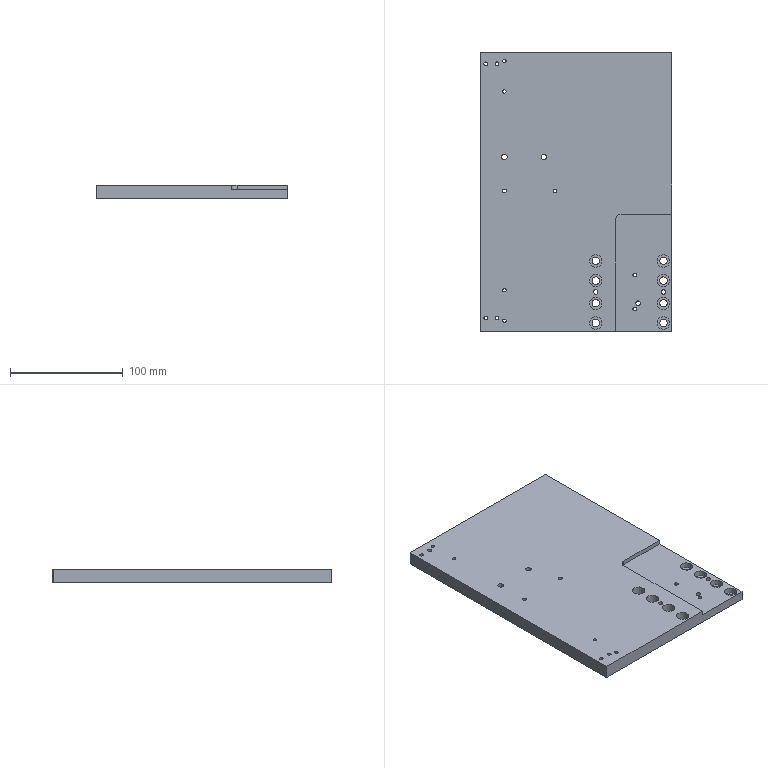CAM job | NX | 3-axis milling, drilling | part box 170 x 247.2 x 12 mm | stock box 170 x 247.2 x 12 mm
Tools:
number,name,description,diameter,corner_radius,flute_length,length,flutes
6,D6,平底铣刀-粗,6.0,0.0,25.0,75.0,2
9,D10,平底铣刀-粗,10.0,0.0,35.0,75.0,2
7,D6-J,平底铣刀-精,6.0,0.0,25.0,75.0,2
10,D10-J,平底铣刀-精,10.0,0.0,35.0,75.0,2
2,D6倒角刀,倒角刀,6.0,0.0,3.0,25.0,2
21,M4X0.7,丝锥,3.3,0.0,35.0,50.0,2
11,D3铰刀,Drilling Tool,3.0,0.0,75.0,100.0,6
23,D4铰刀,Drilling Tool,4.0,0.0,75.0,100.0,6
24,D5铰刀,Drilling Tool,5.0,0.0,75.0,100.0,6
1,C6定点钻,倒角刀,6.0,0.0,3.0,3.0,2
13,ZT3.4,钻头,3.4,0.0,35.0,50.0,2
20,钻头6.6,Drilling Tool,6.6,0.0,35.0,50.0,2
17,ZT2.9,Drilling Tool,2.9,0.0,35.0,50.0,2
18,ZT3.9,Drilling Tool,3.9,0.0,35.0,50.0,2
19,ZT4.9,Drilling Tool,4.9,0.0,35.0,50.0,2
Operations:
program,operation,operation_type,tool,method,geometry_group,spindle_rpm,surface_speed,feed_per_tooth,feed_cut,feed_plunge,cut_length_mm,path_length_mm,cut_time_min,machine_time_min
B,DRILL_CHAMFER_4,Operation,D6倒角刀,METHOD,W-B,2000.0,0.0,0.025,100.0,0.0,19.2,317.958,0.192,0.2219
B,DRILL_CHAMFER_5,Operation,D6倒角刀,METHOD,W-B,2000.0,0.0,0.025,100.0,0.0,15.9,141.53,0.159,0.1716
B,DRILL_CHAMFER_6,Operation,D6倒角刀,METHOD,W-B,2000.0,0.0,0.025,100.0,0.0,41.6,578.142,0.416,0.4697
B,MILL_CHAMFER_1,PlanarMilling,D6倒角刀,METHOD,W-B,4000.0,75.398,0.075,600.0,100.0,21.936,141.338,0.0366,0.0485
B,MILL_CHAMFER_2,PlanarMilling,D6倒角刀,METHOD,W-B,4000.0,75.398,0.075,600.0,100.0,155.528,663.158,0.2592,0.31
B,C0.3_CLOSEDCONTOUR_CHAMFER6X45L_COPY,PlanarMilling,D6倒角刀,CLIMB_CHAMFER-DEPTH0-STEPG,W-B,4000.0,75.398,0.125,1000.0,100.0,853.899,890.199,0.8539,0.8575
A,FLOORWALL_LAYER_ROUGH-MID_COPY,VolumeBased25DMillingOperation,D10,LAYER_ROUGH-DEPTHK-STEPG,W-A,3000.0,94.248,0.5,3000.0,100.0,15338.403,16825.457,5.113,5.261
A,SPOT_DEPTH0.8,Operation,C6定点钻,NONE,W-A,3000.0,56.0,0.01,60.0,90.0,45.0,790.788,0.75,0.8246
A,THRU_PRECISION3.0_PREDRILL,Operation,ZT2.9,NONE,W-A,2000.0,18.221,0.0088,35.0,90.0,67.349,407.937,1.924,1.958
A,THRU_PRECISION4.0_PREDRILL,Operation,ZT3.9,NONE,W-A,1500.0,18.378,0.0167,50.0,90.0,43.578,196.816,0.8715,0.8869
A,THRU_M4_TAPDRILL,Operation,ZT3.4,NONE,W-A,1500.0,15.551,0.02,60.0,90.0,144.0,767.975,2.4,2.462
A,THRU_PRECISION6.0_PREDRILL,Operation,ZT4.9,NONE,W-A,1000.0,15.394,0.03,60.0,90.0,34.829,145.672,0.5805,0.5916
A,COUNTERBORE_DRILL_SEG0,Operation,钻头6.6,NONE,W-A,600.0,12.441,0.1,120.0,90.0,119.642,460.418,0.997,1.031
A,HOLE_ROUGH_D6_1,CylinderMilling,D6,NONE,W-A,4000.0,75.398,0.25,2000.0,100.0,2955.862,3222.362,1.478,1.505
A,HOLE_ROUGH_D6_2,CylinderMilling,D6,NONE,W-A,4000.0,75.398,0.25,2000.0,100.0,1779.547,2044.147,0.8898,0.9162
A,HOLE_FINISH_D6_1,CylinderMilling,D6-J,FINISH_STEPDEPTH_OFF,W-A,4000.0,75.398,0.1,800.0,100.0,212.749,481.249,0.2659,0.2928
A,HOLE_FINISH_D6_2,CylinderMilling,D6-J,FINISH_STEPDEPTH_OFF,W-A,4000.0,75.398,0.1,800.0,100.0,161.317,427.917,0.2016,0.2283
A,DRILL_CHAMFER_1,Operation,D6倒角刀,METHOD,W-A,4000.0,75.398,0.01,80.0,0.0,19.2,317.958,0.24,0.2699
A,DRILL_CHAMFER_2,Operation,D6倒角刀,METHOD,W-A,4000.0,75.398,0.01,80.0,0.0,41.6,578.297,0.52,0.5737
A,DRILL_CHAMFER_3,Operation,D6倒角刀,METHOD,W-A,4000.0,75.398,0.01,80.0,0.0,15.9,145.923,0.1987,0.2118
A,PLANE_DEBURR6X45L_COPY,SurfaceContour,D6倒角刀,CLIMB_CHAMFER-DEPTH0-STEPG,W-A,3500.0,65.972,0.1429,1000.0,100.0,1406.24,2931.529,1.406,1.559
A,REAM,Operation,D3铰刀,METHOD,W-A,500.0,4.712,0.0167,50.0,0.0,56.0,385.24,1.12,1.153
A,REAM_2,Operation,D4铰刀,METHOD,W-A,500.0,6.283,0.0167,50.0,0.0,42.0,189.466,0.84,0.8547
A,REAM_3,Operation,D5铰刀,METHOD,W-A,500.0,7.854,0.0167,50.0,0.0,28.0,132.014,0.56,0.5704
A,THRU_TAP_M4,Operation,M4X0.7,METHOD,W-A,500.0,5.184,0.0007,0.7,90.0,132.0,743.832,188.571,188.633
A,FLOORWALL_FINISH_BOTTOM-MID_COPY,VolumeBased25DMillingOperation,D10-J,FINISH_STEPDEPTH_OFF,W-A,3000.0,94.248,0.1667,1000.0,100.0,1051.459,1077.059,1.052,1.054
A,FLOORWALL_FINISH_SIDE-MID-SELBOTTOM_COPY,VolumeBased25DMillingOperation,D10-J,SIDEMILL_FINISH-DEPTHK-STEPG,W-A,3000.0,94.248,0.1667,1000.0,100.0,162.581,188.381,0.1626,0.1652